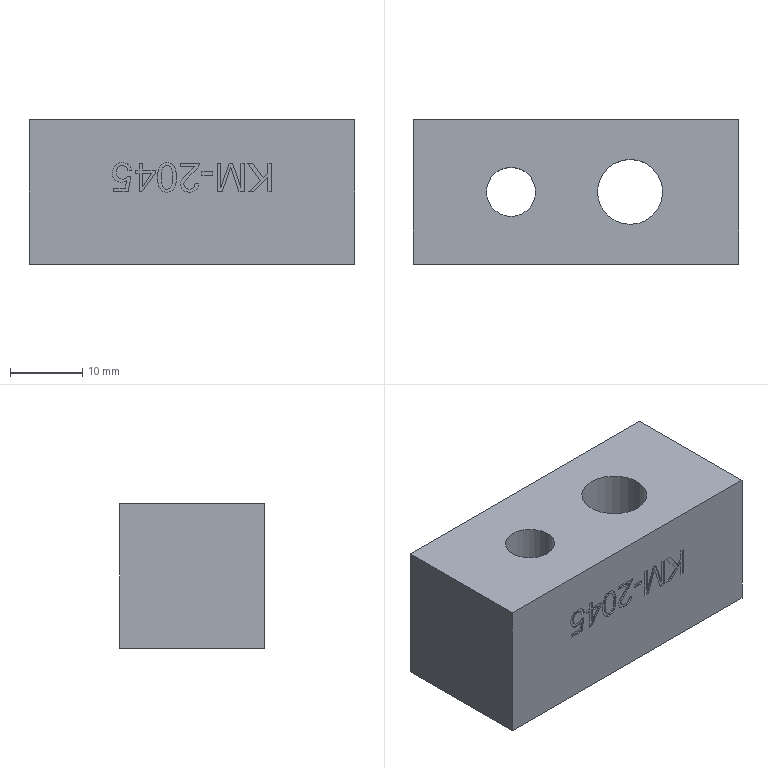Part | NX | features solid 2 | 1 solid | 85 faces | box 45 x 20 x 20 mm | volume 14874 mm3 | plane 69 | spline 12 | cylinder 4 | commonest cylinder face diameters 9 x2 6.8 x1 14 x1